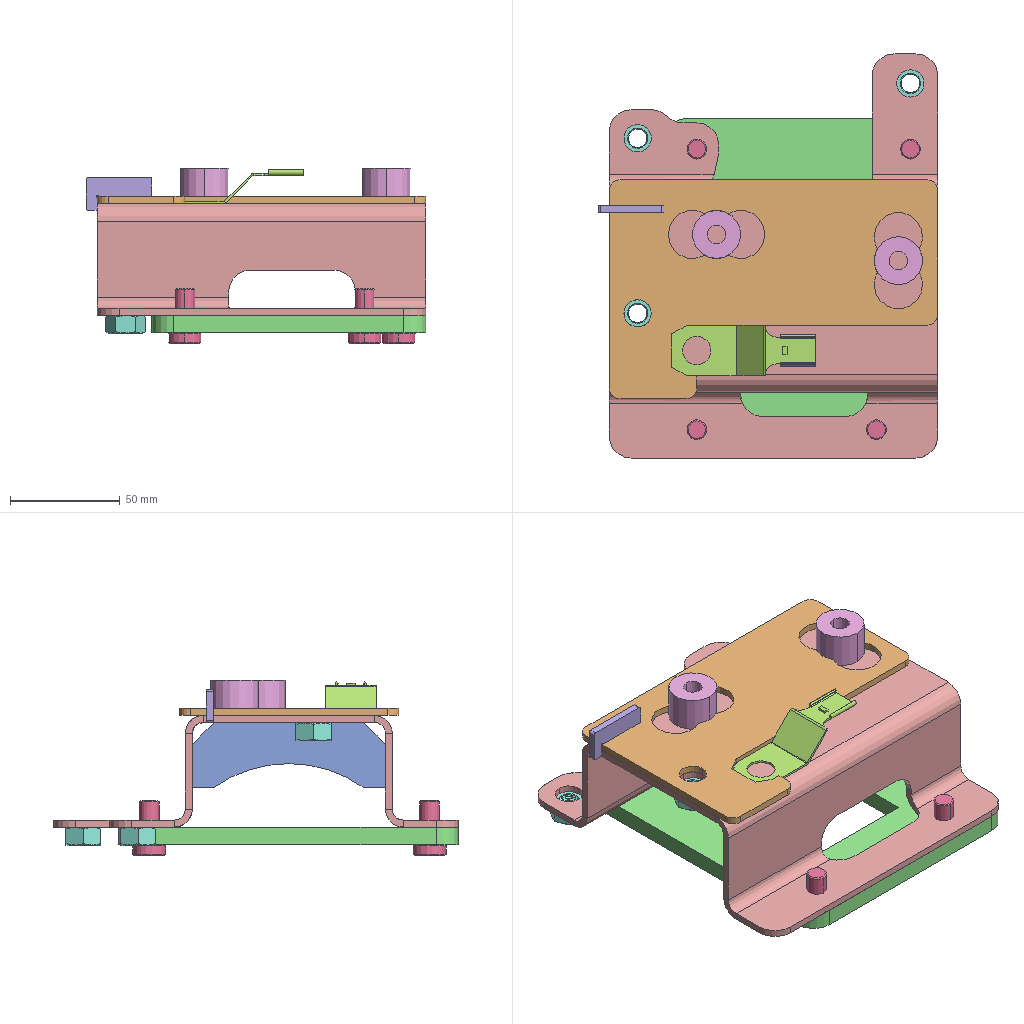Assembly | SolidWorks | 10 different items | 16 placed | box 155 x 185 x 80 mm
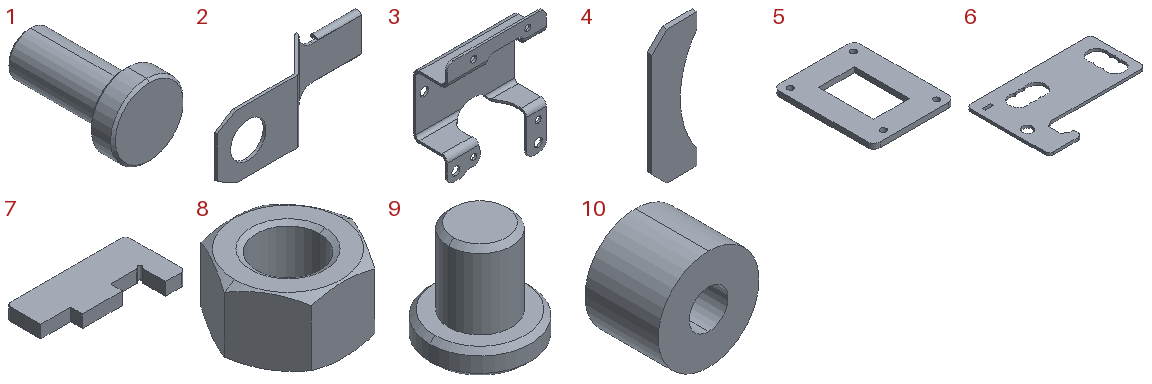Parts list (item | quantity | size | volume | features):
1 | x4 | 15 x 25 x 15 mm | 2141 mm3 | features Chamfer 1, Revolution 1
2 | x1 | 65.7 x 15.573 x 23.06 mm | 1342 mm3 | features BaseBody 1
3 | x1 | 150 x 51 x 184.5 mm | 92629 mm3 | features ICE 2, Fillet 1, FlatPattern 1, Fold 1, SMBaseFlange 1, SheetMetal 1, UnFold 1
4 | x1 | 29.8 x 3.2 x 88.1 mm | 6438 mm3 | features FlatPattern 1, SMBaseFlange 1, SheetMetal 1
5 | x1 | 125 x 155 x 8 mm | 114878 mm3 | features FlatPattern 1, SMBaseFlange 1, SheetMetal 1
6 | x1 | 150 x 100 x 3.2 mm | 29466 mm3 | features FlatPattern 1, SMBaseFlange 1, SheetMetal 1
7 | x1 | 30 x 15 x 3.2 mm | 1020 mm3 | features FlatPattern 1, SMBaseFlange 1, SheetMetal 1
8 | x3 | 27.713 x 24 x 14.8 mm | 5071 mm3 | features RevCut 2, Chamfer 1, Extrusion 1, LPattern 1
9 | x1 | 20 x 20 x 20 mm | 3332 mm3 | features Chamfer 1, Revolution 1
10 | x2 | 22 x 16 x 22 mm | 5174 mm3 | features Extrusion 1, HoleWzd 1
Mates (type | each side: item.copy, entity, surface, feature):
Coincident | 3.1 face plane Base-Flange1 | 4.1 face plane Base-Flange1 | 2 times
DistanceDim | 4.1 face plane Base-Flange1 | 3.1 face plane Base-Flange1
Coincident | 3.1 face plane Base-Flange1 | 2.1 face plane Input1
DistanceDim | 2.1 face cylinder Input1 | 3.1 face plane Base-Flange1 | 2 times
Parallel | 3.1 face plane Base-Flange1 | 2.1 face plane Input1
Coincident | 3.1 face plane Base-Flange1 | 10.1 face plane Boss-Extrude1
DistanceDim | 10.1 face cylinder Boss-Extrude1 | 3.1 face plane Base-Flange1 | 2 times
Parallel | 3.1 face plane Base-Flange1 | 10.1 plane
Coincident | 3.1 face plane Base-Flange1 | 10.2 face plane Boss-Extrude1
DistanceDim | 10.2 face cylinder Boss-Extrude1 | 3.1 face plane Base-Flange1 | 2 times
Parallel | 3.1 face plane Base-Flange1 | 10.2 plane
Concentric | 3.1 face cylinder Cut-Extrude2 | 8.1 face cone EndChamfer
Coincident | 3.1 face plane Base-Flange1 | 8.1 face plane BaseNut
Concentric | 3.1 face cylinder Cut-Extrude2 | 8.2 face cone EndChamfer
Coincident | 3.1 face plane Base-Flange1 | 8.2 face plane BaseNut
Concentric | 3.1 face cylinder Cut-Extrude2 | 8.3 face cone EndChamfer
Coincident | 3.1 face plane Base-Flange1 | 8.3 face plane BaseNut
Parallel | 3.1 face plane Base-Flange1 | 8.1 face plane BaseNut
Parallel | 3.1 face plane Cut-Extrude1 | 8.2 face plane BaseNut
Parallel | 3.1 face plane Cut-Extrude1 | 8.3 face plane BaseNut
InPlace | 3.1 face plane Base-Flange1 | 6.1 plane
Coincident | 6.1 face plane Base-Flange1 | 7.1 face plane Base-Flange1 | 2 times
DistanceDim | 7.1 face plane Base-Flange1 | 6.1 face plane Base-Flange1
InPlace | 3.1 face plane Base-Flange1 | 5.1 plane
Concentric | 5.1 face cylinder Base-Flange1 | 1.1 face cylinder Revolve1
Coincident | 5.1 face plane Base-Flange1 | 1.1 face plane Revolve1
Concentric | 5.1 face cylinder Base-Flange1 | 1.2 face cylinder Revolve1
Coincident | 5.1 face plane Base-Flange1 | 1.2 face plane Revolve1
Concentric | 5.1 face cylinder Base-Flange1 | 1.3 face cylinder Revolve1
Coincident | 5.1 face plane Base-Flange1 | 1.3 face plane Revolve1
Concentric | 5.1 face cylinder Base-Flange1 | 1.4 face cylinder Revolve1
Coincident | 5.1 face plane Base-Flange1 | 1.4 face plane Revolve1